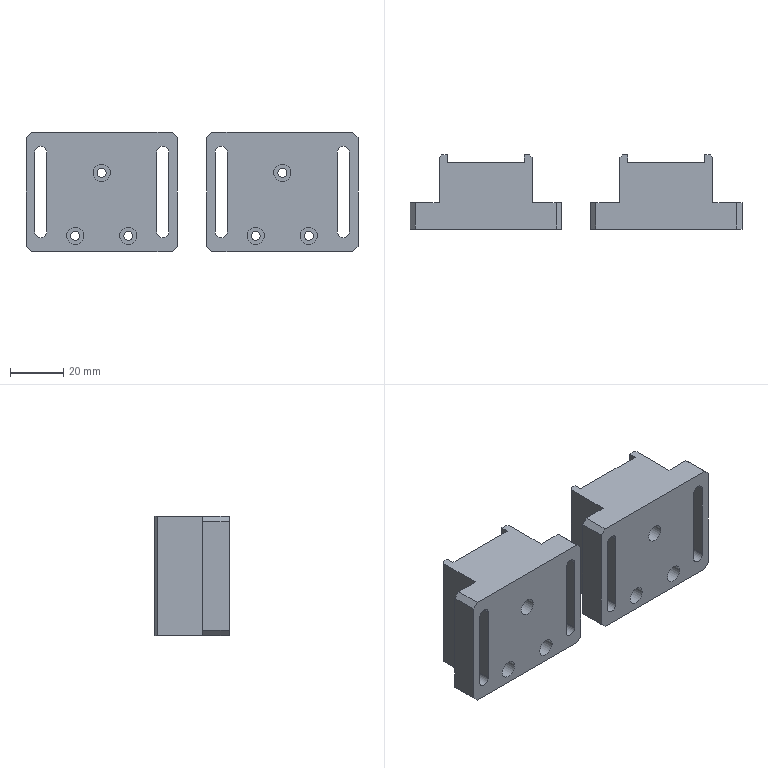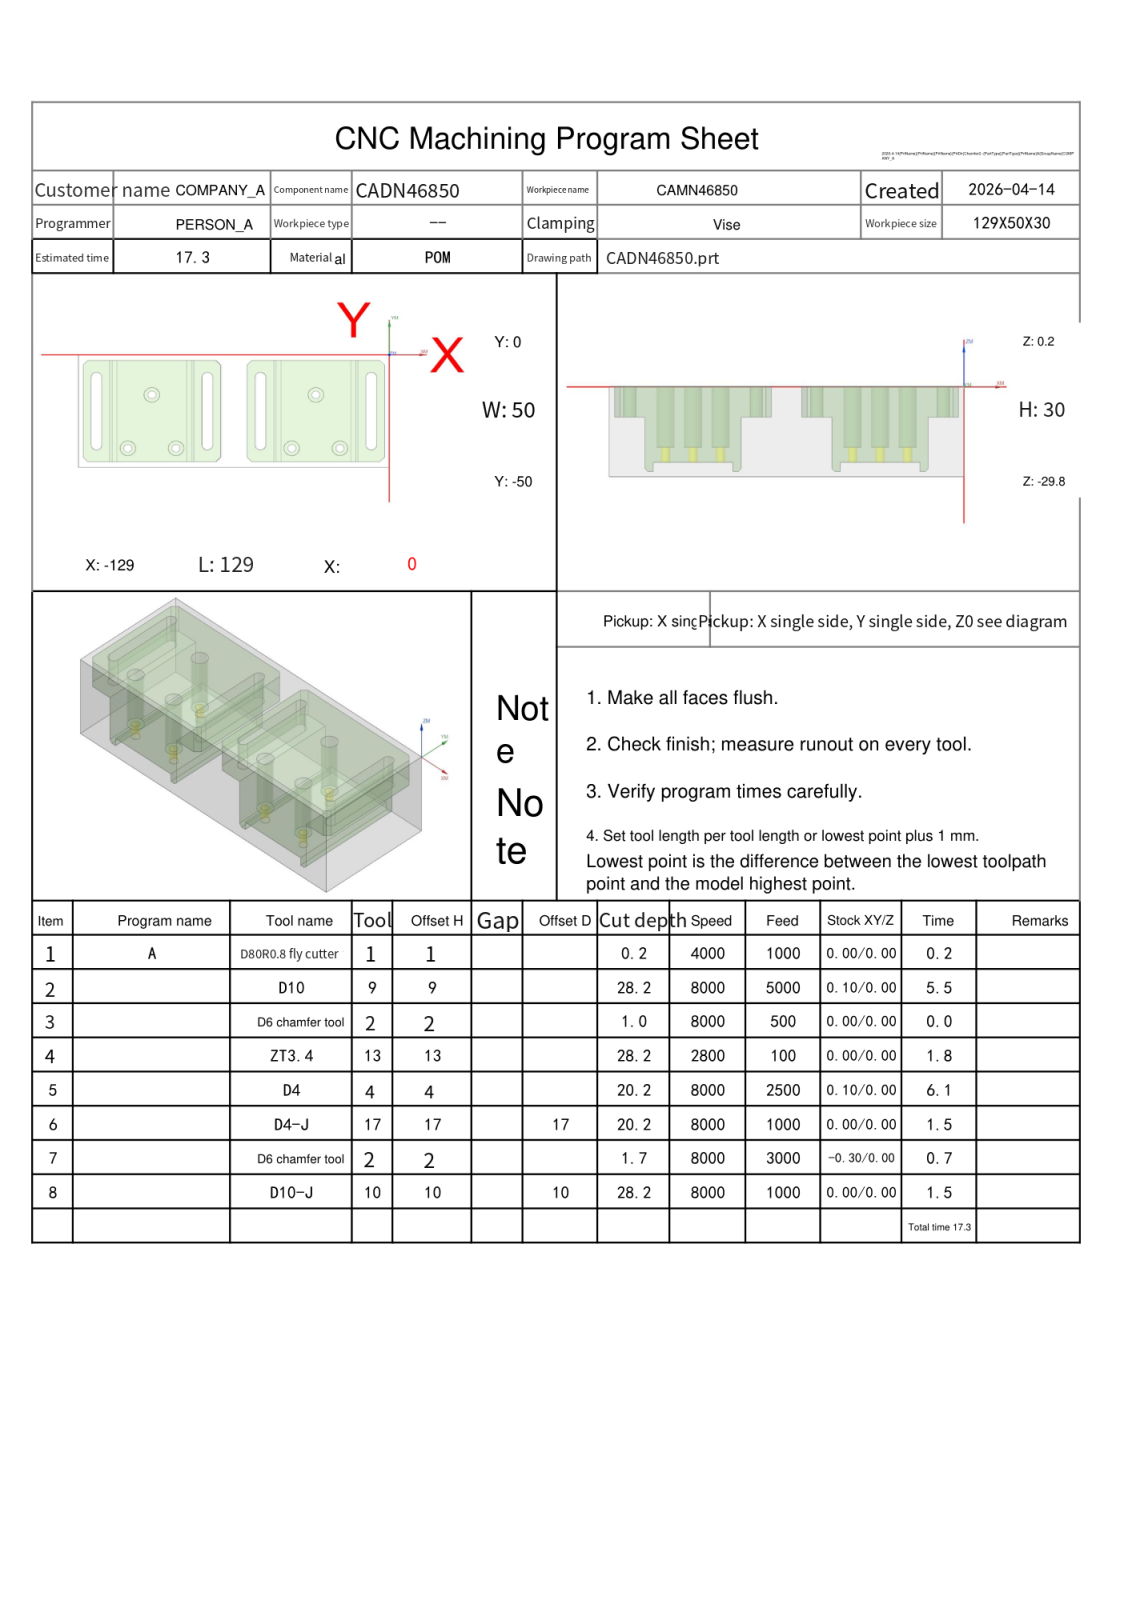NC program | NX | posted by the shop | part box 125 x 28 x 45 mm
Lines 1945 to 1996 of 4607:
N3 T02 M06
(D6 chamfer tool  D=6. R=0. H=02 ce=0.00 di=0.00)
G00 G90 G54 X-30.5 Y-17.8 M03 S8000
G43 H02 Z20.
M08
G98 G81 X-30.5 Y-17.8 Z-.8 R1. F500.
X-20.5 Y-41.5
X-40.5
X-88.5
X-108.5
X-98.5 Y-17.8
X-121.5 Y-10.
Y-40.
X-75.5 Y-10.
Y-40.
X-53.5 Y-10.
Y-40.
X-7.5 Y-10.
Y-40.
G80
G00 Z20.
G91 G28 Z0.0
M05
M09
G91 G28 Z0.0
M01
N4 T13 M06
(ZT3.4 D=3.4 DR_a=118 H=13)
G00 G90 G54 X-30.5 Y-17.8 M03 S2800
G43 H13 Z20.
M08
G98 G83 X-30.5 Y-17.8 Z-28.021 R1. F300. Q2.
X-20.5 Y-41.5
X-40.5
X-88.5
X-108.5
X-98.5 Y-17.8
G98 G83 X-121.5 Y-10. Z-13.021 R1. Q2.
Y-40.
X-75.5
Y-10.
X-53.5
Y-40.
X-7.5 Y-10.
Y-40.
G80
G00 Z20.
G91 G28 Z0.0
M05
M09
G91 G28 Z0.0
M01